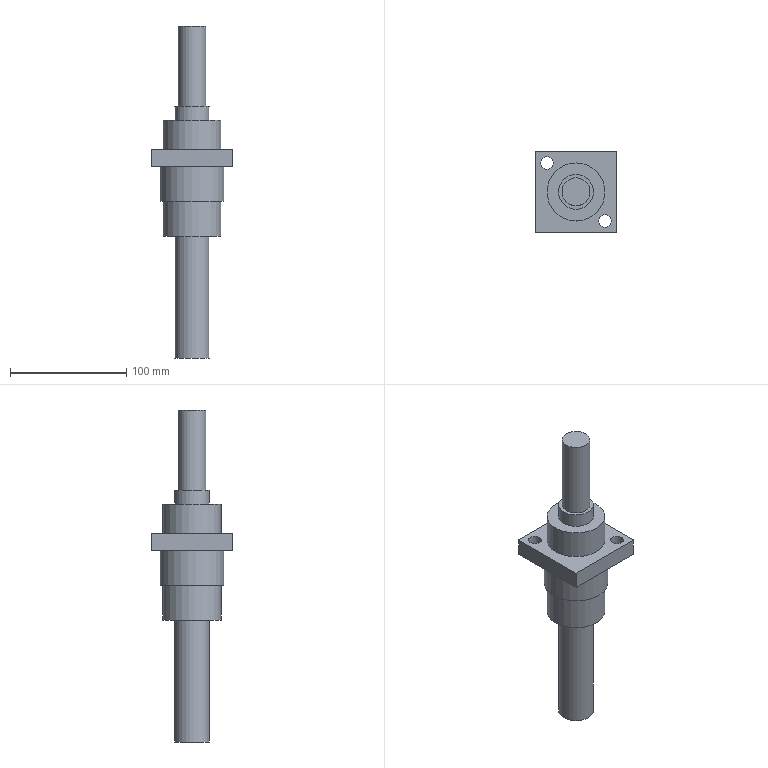Part | NX | features solid 2 | 1 solid | 20 faces | box 70 x 70 x 286 mm | volume 363833 mm3 | plane 12 | cylinder 8 | commonest cylinder face diameters 11 x2 30 x2 50 x2 24 x1 55 x1
STEP:
#1=CARTESIAN_POINT('',(652.5,-225.,-93.));
#2=VERTEX_POINT('',#1);
#3=CARTESIAN_POINT('',(652.5,-210.,-93.));
#4=DIRECTION('',(0.,0.,1.));
#5=DIRECTION('',(0.,-1.,0.));
#6=AXIS2_PLACEMENT_3D('',#3,#4,#5);
#7=CIRCLE('',#6,15.);
#8=EDGE_CURVE('',#2,#2,#7,.T.);
#9=ORIENTED_EDGE('',*,*,#8,.T.);
#10=EDGE_LOOP('',(#9));
#11=FACE_BOUND('',#10,.T.);
#12=CARTESIAN_POINT('',(652.5,-222.,-93.));
#13=VERTEX_POINT('',#12);
#14=CARTESIAN_POINT('',(652.5,-210.,-93.));
#15=DIRECTION('',(0.,0.,1.));
#16=DIRECTION('',(0.,-1.,0.));
#17=AXIS2_PLACEMENT_3D('',#14,#15,#16);
#18=CIRCLE('',#17,12.);
#19=EDGE_CURVE('',#13,#13,#18,.F.);
#20=ORIENTED_EDGE('',*,*,#19,.T.);
#21=EDGE_LOOP('',(#20));
#22=FACE_BOUND('',#21,.T.);
#23=CARTESIAN_POINT('',(652.5,-210.,-93.));
#24=DIRECTION('',(0.,0.,-1.));
#25=DIRECTION('',(0.,-1.,0.));
#26=AXIS2_PLACEMENT_3D('',#23,#24,#25);
#27=PLANE('',#26);
#28=ADVANCED_FACE('',(#11,#22),#27,.F.);
#29=CARTESIAN_POINT('',(627.5,-190.5,-130.));
#30=VERTEX_POINT('',#29);
#31=CARTESIAN_POINT('',(627.5,-185.,-130.));
#32=DIRECTION('',(0.,0.,1.));
#33=DIRECTION('',(0.,-1.,0.));
#34=AXIS2_PLACEMENT_3D('',#31,#32,#33);
#35=CIRCLE('',#34,5.5);
#36=EDGE_CURVE('',#30,#30,#35,.T.);
#37=ORIENTED_EDGE('',*,*,#36,.F.);
#38=EDGE_LOOP('',(#37));
#39=FACE_BOUND('',#38,.T.);
#40=CARTESIAN_POINT('',(677.5,-240.5,-130.));
#41=VERTEX_POINT('',#40);
#42=CARTESIAN_POINT('',(677.5,-235.,-130.));
#43=DIRECTION('',(0.,0.,1.));
#44=DIRECTION('',(0.,-1.,0.));
#45=AXIS2_PLACEMENT_3D('',#42,#43,#44);
#46=CIRCLE('',#45,5.5);
#47=EDGE_CURVE('',#41,#41,#46,.T.);
#48=ORIENTED_EDGE('',*,*,#47,.F.);
#49=EDGE_LOOP('',(#48));
#50=FACE_BOUND('',#49,.T.);
#51=CARTESIAN_POINT('',(687.5,-175.,-130.));
#52=VERTEX_POINT('',#51);
#53=CARTESIAN_POINT('',(617.5,-175.,-130.));
#54=VERTEX_POINT('',#53);
#55=CARTESIAN_POINT('',(687.5,-175.,-130.));
#56=DIRECTION('',(-1.,0.,0.));
#57=VECTOR('',#56,1000.);
#58=LINE('',#55,#57);
#59=EDGE_CURVE('',#52,#54,#58,.T.);
#60=ORIENTED_EDGE('',*,*,#59,.T.);
#61=CARTESIAN_POINT('',(617.5,-245.,-130.));
#62=VERTEX_POINT('',#61);
#63=CARTESIAN_POINT('',(617.5,-175.,-130.));
#64=DIRECTION('',(0.,-1.,0.));
#65=VECTOR('',#64,1000.);
#66=LINE('',#63,#65);
#67=EDGE_CURVE('',#54,#62,#66,.T.);
#68=ORIENTED_EDGE('',*,*,#67,.T.);
#69=CARTESIAN_POINT('',(687.5,-245.,-130.));
#70=VERTEX_POINT('',#69);
#71=CARTESIAN_POINT('',(617.5,-245.,-130.));
#72=DIRECTION('',(1.,0.,0.));
#73=VECTOR('',#72,1000.);
#74=LINE('',#71,#73);
#75=EDGE_CURVE('',#62,#70,#74,.T.);
#76=ORIENTED_EDGE('',*,*,#75,.T.);
#77=CARTESIAN_POINT('',(687.5,-245.,-130.));
#78=DIRECTION('',(0.,1.,0.));
#79=VECTOR('',#78,1000.);
#80=LINE('',#77,#79);
#81=EDGE_CURVE('',#70,#52,#80,.T.);
#82=ORIENTED_EDGE('',*,*,#81,.T.);
#83=EDGE_LOOP('',(#60,#68,#76,#82));
#84=FACE_BOUND('',#83,.T.);
#85=CARTESIAN_POINT('',(652.5,-185.,-130.));
#86=VERTEX_POINT('',#85);
#87=CARTESIAN_POINT('',(652.5,-210.,-130.));
#88=DIRECTION('',(0.,0.,-1.));
#89=DIRECTION('',(0.,1.,0.));
#90=AXIS2_PLACEMENT_3D('',#87,#88,#89);
#91=CIRCLE('',#90,25.);
#92=EDGE_CURVE('',#86,#86,#91,.F.);
#93=ORIENTED_EDGE('',*,*,#92,.F.);
#94=EDGE_LOOP('',(#93));
#95=FACE_BOUND('',#94,.T.);
#96=CARTESIAN_POINT('',(617.5,-175.,-130.));
#97=DIRECTION('',(0.,0.,1.));
#98=DIRECTION('',(0.,-1.,0.));
#99=AXIS2_PLACEMENT_3D('',#96,#97,#98);
#100=PLANE('',#99);
#101=ADVANCED_FACE('',(#39,#50,#84,#95),#100,.T.);
#102=CARTESIAN_POINT('',(687.5,-175.,-145.));
#103=VERTEX_POINT('',#102);
#104=CARTESIAN_POINT('',(617.5,-175.,-145.));
#105=VERTEX_POINT('',#104);
#106=CARTESIAN_POINT('',(687.5,-175.,-145.));
#107=DIRECTION('',(-1.,0.,0.));
#108=VECTOR('',#107,1000.);
#109=LINE('',#106,#108);
#110=EDGE_CURVE('',#103,#105,#109,.T.);
#111=ORIENTED_EDGE('',*,*,#110,.F.);
#112=CARTESIAN_POINT('',(687.5,-245.,-145.));
#113=VERTEX_POINT('',#112);
#114=CARTESIAN_POINT('',(687.5,-245.,-145.));
#115=DIRECTION('',(0.,1.,0.));
#116=VECTOR('',#115,1000.);
#117=LINE('',#114,#116);
#118=EDGE_CURVE('',#113,#103,#117,.T.);
#119=ORIENTED_EDGE('',*,*,#118,.F.);
#120=CARTESIAN_POINT('',(617.5,-245.,-145.));
#121=VERTEX_POINT('',#120);
#122=CARTESIAN_POINT('',(617.5,-245.,-145.));
#123=DIRECTION('',(1.,0.,0.));
#124=VECTOR('',#123,1000.);
#125=LINE('',#122,#124);
#126=EDGE_CURVE('',#121,#113,#125,.T.);
#127=ORIENTED_EDGE('',*,*,#126,.F.);
#128=CARTESIAN_POINT('',(617.5,-175.,-145.));
#129=DIRECTION('',(0.,-1.,0.));
#130=VECTOR('',#129,1000.);
#131=LINE('',#128,#130);
#132=EDGE_CURVE('',#105,#121,#131,.T.);
#133=ORIENTED_EDGE('',*,*,#132,.F.);
#134=EDGE_LOOP('',(#111,#119,#127,#133));
#135=FACE_BOUND('',#134,.T.);
#136=CARTESIAN_POINT('',(677.5,-240.5,-145.));
#137=VERTEX_POINT('',#136);
#138=CARTESIAN_POINT('',(677.5,-235.,-145.));
#139=DIRECTION('',(0.,0.,1.));
#140=DIRECTION('',(0.,-1.,0.));
#141=AXIS2_PLACEMENT_3D('',#138,#139,#140);
#142=CIRCLE('',#141,5.5);
#143=EDGE_CURVE('',#137,#137,#142,.T.);
#144=ORIENTED_EDGE('',*,*,#143,.T.);
#145=EDGE_LOOP('',(#144));
#146=FACE_BOUND('',#145,.T.);
#147=CARTESIAN_POINT('',(627.5,-190.5,-145.));
#148=VERTEX_POINT('',#147);
#149=CARTESIAN_POINT('',(627.5,-185.,-145.));
#150=DIRECTION('',(0.,0.,1.));
#151=DIRECTION('',(0.,-1.,0.));
#152=AXIS2_PLACEMENT_3D('',#149,#150,#151);
#153=CIRCLE('',#152,5.5);
#154=EDGE_CURVE('',#148,#148,#153,.T.);
#155=ORIENTED_EDGE('',*,*,#154,.T.);
#156=EDGE_LOOP('',(#155));
#157=FACE_BOUND('',#156,.T.);
#158=CARTESIAN_POINT('',(652.5,-182.5,-145.));
#159=VERTEX_POINT('',#158);
#160=CARTESIAN_POINT('',(652.5,-210.,-145.));
#161=DIRECTION('',(0.,0.,-1.));
#162=DIRECTION('',(0.,1.,0.));
#163=AXIS2_PLACEMENT_3D('',#160,#161,#162);
#164=CIRCLE('',#163,27.5);
#165=EDGE_CURVE('',#159,#159,#164,.F.);
#166=ORIENTED_EDGE('',*,*,#165,.T.);
#167=EDGE_LOOP('',(#166));
#168=FACE_BOUND('',#167,.T.);
#169=CARTESIAN_POINT('',(617.5,-175.,-145.));
#170=DIRECTION('',(0.,0.,1.));
#171=DIRECTION('',(0.,-1.,0.));
#172=AXIS2_PLACEMENT_3D('',#169,#170,#171);
#173=PLANE('',#172);
#174=ADVANCED_FACE('',(#135,#146,#157,#168),#173,.F.);
#175=ORIENTED_EDGE('',*,*,#59,.F.);
#176=CARTESIAN_POINT('',(687.5,-175.,-145.));
#177=DIRECTION('',(0.,0.,1.));
#178=VECTOR('',#177,1000.);
#179=LINE('',#176,#178);
#180=EDGE_CURVE('',#103,#52,#179,.T.);
#181=ORIENTED_EDGE('',*,*,#180,.F.);
#182=ORIENTED_EDGE('',*,*,#110,.T.);
#183=CARTESIAN_POINT('',(617.5,-175.,-145.));
#184=DIRECTION('',(0.,0.,1.));
#185=VECTOR('',#184,1000.);
#186=LINE('',#183,#185);
#187=EDGE_CURVE('',#105,#54,#186,.T.);
#188=ORIENTED_EDGE('',*,*,#187,.T.);
#189=EDGE_LOOP('',(#175,#181,#182,#188));
#190=FACE_BOUND('',#189,.T.);
#191=CARTESIAN_POINT('',(687.5,-175.,-145.));
#192=DIRECTION('',(0.,1.,0.));
#193=DIRECTION('',(0.,0.,1.));
#194=AXIS2_PLACEMENT_3D('',#191,#192,#193);
#195=PLANE('',#194);
#196=ADVANCED_FACE('',(#190),#195,.T.);
#197=ORIENTED_EDGE('',*,*,#67,.F.);
#198=ORIENTED_EDGE('',*,*,#187,.F.);
#199=ORIENTED_EDGE('',*,*,#132,.T.);
#200=CARTESIAN_POINT('',(617.5,-245.,-145.));
#201=DIRECTION('',(0.,0.,1.));
#202=VECTOR('',#201,1000.);
#203=LINE('',#200,#202);
#204=EDGE_CURVE('',#121,#62,#203,.T.);
#205=ORIENTED_EDGE('',*,*,#204,.T.);
#206=EDGE_LOOP('',(#197,#198,#199,#205));
#207=FACE_BOUND('',#206,.T.);
#208=CARTESIAN_POINT('',(617.5,-175.,-145.));
#209=DIRECTION('',(-1.,0.,0.));
#210=DIRECTION('',(0.,0.,-1.));
#211=AXIS2_PLACEMENT_3D('',#208,#209,#210);
#212=PLANE('',#211);
#213=ADVANCED_FACE('',(#207),#212,.T.);
#214=ORIENTED_EDGE('',*,*,#75,.F.);
#215=ORIENTED_EDGE('',*,*,#204,.F.);
#216=ORIENTED_EDGE('',*,*,#126,.T.);
#217=CARTESIAN_POINT('',(687.5,-245.,-145.));
#218=DIRECTION('',(0.,0.,1.));
#219=VECTOR('',#218,1000.);
#220=LINE('',#217,#219);
#221=EDGE_CURVE('',#113,#70,#220,.T.);
#222=ORIENTED_EDGE('',*,*,#221,.T.);
#223=EDGE_LOOP('',(#214,#215,#216,#222));
#224=FACE_BOUND('',#223,.T.);
#225=CARTESIAN_POINT('',(617.5,-245.,-145.));
#226=DIRECTION('',(0.,-1.,0.));
#227=DIRECTION('',(0.,0.,-1.));
#228=AXIS2_PLACEMENT_3D('',#225,#226,#227);
#229=PLANE('',#228);
#230=ADVANCED_FACE('',(#224),#229,.T.);
#231=ORIENTED_EDGE('',*,*,#143,.F.);
#232=EDGE_LOOP('',(#231));
#233=FACE_BOUND('',#232,.T.);
#234=ORIENTED_EDGE('',*,*,#47,.T.);
#235=EDGE_LOOP('',(#234));
#236=FACE_BOUND('',#235,.T.);
#237=CARTESIAN_POINT('',(677.5,-235.,-145.));
#238=DIRECTION('',(0.,0.,1.));
#239=DIRECTION('',(0.,-1.,0.));
#240=AXIS2_PLACEMENT_3D('',#237,#238,#239);
#241=CYLINDRICAL_SURFACE('',#240,5.5);
#242=ADVANCED_FACE('',(#233,#236),#241,.F.);
#243=ORIENTED_EDGE('',*,*,#154,.F.);
#244=EDGE_LOOP('',(#243));
#245=FACE_BOUND('',#244,.T.);
#246=ORIENTED_EDGE('',*,*,#36,.T.);
#247=EDGE_LOOP('',(#246));
#248=FACE_BOUND('',#247,.T.);
#249=CARTESIAN_POINT('',(627.5,-185.,-145.));
#250=DIRECTION('',(0.,0.,1.));
#251=DIRECTION('',(0.,-1.,0.));
#252=AXIS2_PLACEMENT_3D('',#249,#250,#251);
#253=CYLINDRICAL_SURFACE('',#252,5.5);
#254=ADVANCED_FACE('',(#245,#248),#253,.F.);
#255=ORIENTED_EDGE('',*,*,#81,.F.);
#256=ORIENTED_EDGE('',*,*,#221,.F.);
#257=ORIENTED_EDGE('',*,*,#118,.T.);
#258=ORIENTED_EDGE('',*,*,#180,.T.);
#259=EDGE_LOOP('',(#255,#256,#257,#258));
#260=FACE_BOUND('',#259,.T.);
#261=CARTESIAN_POINT('',(687.5,-245.,-145.));
#262=DIRECTION('',(1.,0.,0.));
#263=DIRECTION('',(0.,0.,1.));
#264=AXIS2_PLACEMENT_3D('',#261,#262,#263);
#265=PLANE('',#264);
#266=ADVANCED_FACE('',(#260),#265,.T.);
#267=CARTESIAN_POINT('',(652.5,-182.5,-175.));
#268=VERTEX_POINT('',#267);
#269=CARTESIAN_POINT('',(652.5,-210.,-175.));
#270=DIRECTION('',(0.,0.,-1.));
#271=DIRECTION('',(0.,1.,0.));
#272=AXIS2_PLACEMENT_3D('',#269,#270,#271);
#273=CIRCLE('',#272,27.5);
#274=EDGE_CURVE('',#268,#268,#273,.F.);
#275=ORIENTED_EDGE('',*,*,#274,.F.);
#276=EDGE_LOOP('',(#275));
#277=FACE_BOUND('',#276,.T.);
#278=CARTESIAN_POINT('',(652.5,-235.,-175.));
#279=VERTEX_POINT('',#278);
#280=CARTESIAN_POINT('',(652.5,-210.,-175.));
#281=DIRECTION('',(0.,0.,1.));
#282=DIRECTION('',(0.,-1.,0.));
#283=AXIS2_PLACEMENT_3D('',#280,#281,#282);
#284=CIRCLE('',#283,25.);
#285=EDGE_CURVE('',#279,#279,#284,.T.);
#286=ORIENTED_EDGE('',*,*,#285,.T.);
#287=EDGE_LOOP('',(#286));
#288=FACE_BOUND('',#287,.T.);
#289=CARTESIAN_POINT('',(652.5,-210.,-175.));
#290=DIRECTION('',(0.,0.,-1.));
#291=DIRECTION('',(0.,1.,0.));
#292=AXIS2_PLACEMENT_3D('',#289,#290,#291);
#293=PLANE('',#292);
#294=ADVANCED_FACE('',(#277,#288),#293,.T.);
#295=ORIENTED_EDGE('',*,*,#274,.T.);
#296=EDGE_LOOP('',(#295));
#297=FACE_BOUND('',#296,.T.);
#298=ORIENTED_EDGE('',*,*,#165,.F.);
#299=EDGE_LOOP('',(#298));
#300=FACE_BOUND('',#299,.T.);
#301=CARTESIAN_POINT('',(652.5,-210.,-145.));
#302=DIRECTION('',(0.,0.,-1.));
#303=DIRECTION('',(0.,1.,0.));
#304=AXIS2_PLACEMENT_3D('',#301,#302,#303);
#305=CYLINDRICAL_SURFACE('',#304,27.5);
#306=ADVANCED_FACE('',(#297,#300),#305,.T.);
#307=CARTESIAN_POINT('',(652.5,-235.,-205.));
#308=VERTEX_POINT('',#307);
#309=CARTESIAN_POINT('',(652.5,-210.,-205.));
#310=DIRECTION('',(0.,0.,1.));
#311=DIRECTION('',(0.,-1.,0.));
#312=AXIS2_PLACEMENT_3D('',#309,#310,#311);
#313=CIRCLE('',#312,25.);
#314=EDGE_CURVE('',#308,#308,#313,.T.);
#315=ORIENTED_EDGE('',*,*,#314,.F.);
#316=EDGE_LOOP('',(#315));
#317=FACE_BOUND('',#316,.T.);
#318=CARTESIAN_POINT('',(652.5,-195.,-205.));
#319=VERTEX_POINT('',#318);
#320=CARTESIAN_POINT('',(652.5,-210.,-205.));
#321=DIRECTION('',(0.,0.,-1.));
#322=DIRECTION('',(0.,1.,0.));
#323=AXIS2_PLACEMENT_3D('',#320,#321,#322);
#324=CIRCLE('',#323,15.);
#325=EDGE_CURVE('',#319,#319,#324,.F.);
#326=ORIENTED_EDGE('',*,*,#325,.T.);
#327=EDGE_LOOP('',(#326));
#328=FACE_BOUND('',#327,.T.);
#329=CARTESIAN_POINT('',(652.5,-210.,-205.));
#330=DIRECTION('',(0.,0.,-1.));
#331=DIRECTION('',(0.,1.,0.));
#332=AXIS2_PLACEMENT_3D('',#329,#330,#331);
#333=PLANE('',#332);
#334=ADVANCED_FACE('',(#317,#328),#333,.T.);
#335=ORIENTED_EDGE('',*,*,#285,.F.);
#336=EDGE_LOOP('',(#335));
#337=FACE_BOUND('',#336,.T.);
#338=ORIENTED_EDGE('',*,*,#314,.T.);
#339=EDGE_LOOP('',(#338));
#340=FACE_BOUND('',#339,.T.);
#341=CARTESIAN_POINT('',(652.5,-210.,-105.));
#342=DIRECTION('',(0.,0.,-1.));
#343=DIRECTION('',(0.,1.,0.));
#344=AXIS2_PLACEMENT_3D('',#341,#342,#343);
#345=CYLINDRICAL_SURFACE('',#344,25.);
#346=ADVANCED_FACE('',(#337,#340),#345,.T.);
#347=ORIENTED_EDGE('',*,*,#92,.T.);
#348=EDGE_LOOP('',(#347));
#349=FACE_BOUND('',#348,.T.);
#350=CARTESIAN_POINT('',(652.5,-235.,-105.));
#351=VERTEX_POINT('',#350);
#352=CARTESIAN_POINT('',(652.5,-210.,-105.));
#353=DIRECTION('',(0.,0.,1.));
#354=DIRECTION('',(0.,-1.,0.));
#355=AXIS2_PLACEMENT_3D('',#352,#353,#354);
#356=CIRCLE('',#355,25.);
#357=EDGE_CURVE('',#351,#351,#356,.T.);
#358=ORIENTED_EDGE('',*,*,#357,.F.);
#359=EDGE_LOOP('',(#358));
#360=FACE_BOUND('',#359,.T.);
#361=CARTESIAN_POINT('',(652.5,-210.,-105.));
#362=DIRECTION('',(0.,0.,-1.));
#363=DIRECTION('',(0.,1.,0.));
#364=AXIS2_PLACEMENT_3D('',#361,#362,#363);
#365=CYLINDRICAL_SURFACE('',#364,25.);
#366=ADVANCED_FACE('',(#349,#360),#365,.T.);
#367=ORIENTED_EDGE('',*,*,#357,.T.);
#368=EDGE_LOOP('',(#367));
#369=FACE_BOUND('',#368,.T.);
#370=CARTESIAN_POINT('',(652.5,-225.,-105.));
#371=VERTEX_POINT('',#370);
#372=CARTESIAN_POINT('',(652.5,-210.,-105.));
#373=DIRECTION('',(0.,0.,1.));
#374=DIRECTION('',(0.,-1.,0.));
#375=AXIS2_PLACEMENT_3D('',#372,#373,#374);
#376=CIRCLE('',#375,15.);
#377=EDGE_CURVE('',#371,#371,#376,.F.);
#378=ORIENTED_EDGE('',*,*,#377,.T.);
#379=EDGE_LOOP('',(#378));
#380=FACE_BOUND('',#379,.T.);
#381=CARTESIAN_POINT('',(652.5,-210.,-105.));
#382=DIRECTION('',(0.,0.,-1.));
#383=DIRECTION('',(0.,1.,0.));
#384=AXIS2_PLACEMENT_3D('',#381,#382,#383);
#385=PLANE('',#384);
#386=ADVANCED_FACE('',(#369,#380),#385,.F.);
#387=ORIENTED_EDGE('',*,*,#325,.F.);
#388=EDGE_LOOP('',(#387));
#389=FACE_BOUND('',#388,.T.);
#390=CARTESIAN_POINT('',(652.5,-225.,-310.));
#391=VERTEX_POINT('',#390);
#392=CARTESIAN_POINT('',(652.5,-210.,-310.));
#393=DIRECTION('',(0.,0.,1.));
#394=DIRECTION('',(0.,-1.,0.));
#395=AXIS2_PLACEMENT_3D('',#392,#393,#394);
#396=CIRCLE('',#395,15.);
#397=EDGE_CURVE('',#391,#391,#396,.T.);
#398=ORIENTED_EDGE('',*,*,#397,.T.);
#399=EDGE_LOOP('',(#398));
#400=FACE_BOUND('',#399,.T.);
#401=CARTESIAN_POINT('',(652.5,-210.,-309.));
#402=DIRECTION('',(0.,0.,1.));
#403=DIRECTION('',(0.,1.,0.));
#404=AXIS2_PLACEMENT_3D('',#401,#402,#403);
#405=CYLINDRICAL_SURFACE('',#404,15.);
#406=ADVANCED_FACE('',(#389,#400),#405,.T.);
#407=ORIENTED_EDGE('',*,*,#397,.F.);
#408=EDGE_LOOP('',(#407));
#409=FACE_BOUND('',#408,.T.);
#410=CARTESIAN_POINT('',(652.5,-210.,-310.));
#411=DIRECTION('',(0.,0.,-1.));
#412=DIRECTION('',(0.,-1.,0.));
#413=AXIS2_PLACEMENT_3D('',#410,#411,#412);
#414=PLANE('',#413);
#415=ADVANCED_FACE('',(#409),#414,.T.);
#416=ORIENTED_EDGE('',*,*,#377,.F.);
#417=EDGE_LOOP('',(#416));
#418=FACE_BOUND('',#417,.T.);
#419=ORIENTED_EDGE('',*,*,#8,.F.);
#420=EDGE_LOOP('',(#419));
#421=FACE_BOUND('',#420,.T.);
#422=CARTESIAN_POINT('',(652.5,-210.,-93.));
#423=DIRECTION('',(0.,0.,-1.));
#424=DIRECTION('',(0.,-1.,0.));
#425=AXIS2_PLACEMENT_3D('',#422,#423,#424);
#426=CYLINDRICAL_SURFACE('',#425,15.);
#427=ADVANCED_FACE('',(#418,#421),#426,.T.);
#428=CARTESIAN_POINT('',(652.5,-198.,-24.));
#429=VERTEX_POINT('',#428);
#430=CARTESIAN_POINT('',(652.5,-210.,-24.));
#431=DIRECTION('',(0.,0.,-1.));
#432=DIRECTION('',(0.,1.,0.));
#433=AXIS2_PLACEMENT_3D('',#430,#431,#432);
#434=CIRCLE('',#433,12.);
#435=EDGE_CURVE('',#429,#429,#434,.T.);
#436=ORIENTED_EDGE('',*,*,#435,.T.);
#437=EDGE_LOOP('',(#436));
#438=FACE_BOUND('',#437,.T.);
#439=ORIENTED_EDGE('',*,*,#19,.F.);
#440=EDGE_LOOP('',(#439));
#441=FACE_BOUND('',#440,.T.);
#442=CARTESIAN_POINT('',(652.5,-210.,-43.));
#443=DIRECTION('',(0.,0.,-1.));
#444=DIRECTION('',(0.,-1.,0.));
#445=AXIS2_PLACEMENT_3D('',#442,#443,#444);
#446=CYLINDRICAL_SURFACE('',#445,12.);
#447=ADVANCED_FACE('',(#438,#441),#446,.T.);
#448=ORIENTED_EDGE('',*,*,#435,.F.);
#449=EDGE_LOOP('',(#448));
#450=FACE_BOUND('',#449,.T.);
#451=CARTESIAN_POINT('',(652.5,-210.,-24.));
#452=DIRECTION('',(0.,0.,1.));
#453=DIRECTION('',(0.,1.,0.));
#454=AXIS2_PLACEMENT_3D('',#451,#452,#453);
#455=PLANE('',#454);
#456=ADVANCED_FACE('',(#450),#455,.T.);
#457=CLOSED_SHELL('',(#28,#101,#174,#196,#213,#230,#242,#254,#266,#294,#306,#334,#346,#366,#386,#406,#415,#427,#447,#456));
#458=MANIFOLD_SOLID_BREP('',#457);
#459=(LENGTH_UNIT()NAMED_UNIT(*)SI_UNIT(.MILLI.,.METRE.));
#460=UNCERTAINTY_MEASURE_WITH_UNIT(LENGTH_MEASURE(0.00001),#459,'','');
#461=(NAMED_UNIT(*)PLANE_ANGLE_UNIT()SI_UNIT($,.RADIAN.));
#462=(NAMED_UNIT(*)SI_UNIT($,.STERADIAN.)SOLID_ANGLE_UNIT());
#463=(GEOMETRIC_REPRESENTATION_CONTEXT(3)GLOBAL_UNCERTAINTY_ASSIGNED_CONTEXT((#460))GLOBAL_UNIT_ASSIGNED_CONTEXT((#459,#461,#462))REPRESENTATION_CONTEXT('',''));
#464=ADVANCED_BREP_SHAPE_REPRESENTATION('',(#458),#463);